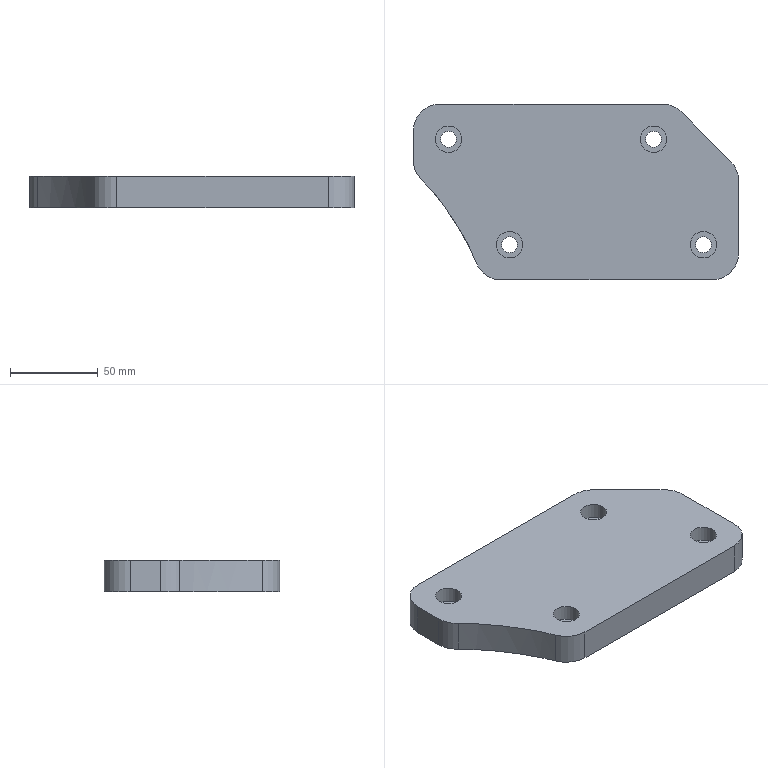Part | STEP file | solid 54 | 1 solid | 26 faces | box 185 x 100 x 18 mm | volume 283727 mm3 | cylinder 14 | plane 11 | spline 1 | commonest cylinder face diameters 30 x6 9 x4 15 x4